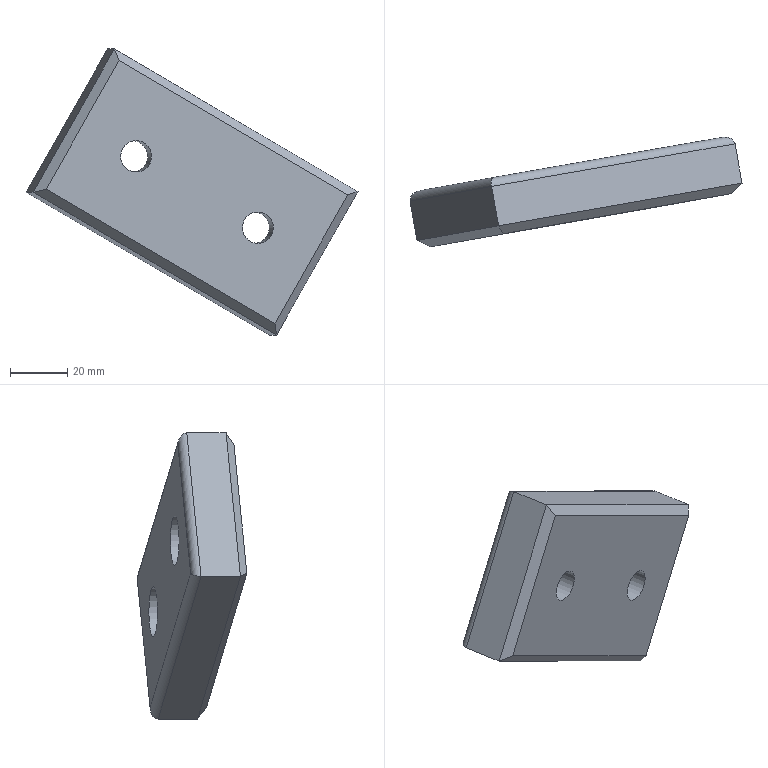Part | NX | features solid 2 | 1 solid | 20 faces | box 116.311 x 38.432 x 100.229 mm | volume 106721 mm3 | plane 12 | cylinder 8 | commonest cylinder face diameters 6 x4 11 x2 17.5 x2
STEP:
#1=CARTESIAN_POINT('',(794.909,638.341,-0.113));
#2=VERTEX_POINT('',#1);
#3=CARTESIAN_POINT('',(792.478,652.128,-0.113));
#4=VERTEX_POINT('',#3);
#5=CARTESIAN_POINT('',(795.43,635.386,-0.113));
#6=DIRECTION('',(-0.1736,0.9848,0.));
#7=VECTOR('',#6,1000.);
#8=LINE('',#5,#7);
#9=EDGE_CURVE('',#2,#4,#8,.T.);
#10=ORIENTED_EDGE('',*,*,#9,.F.);
#11=CARTESIAN_POINT('',(823.469,643.376,50.117));
#12=VERTEX_POINT('',#11);
#13=CARTESIAN_POINT('',(823.469,643.376,50.117));
#14=DIRECTION('',(0.4924,0.08682,0.866));
#15=VECTOR('',#14,1000.);
#16=LINE('',#13,#15);
#17=EDGE_CURVE('',#2,#12,#16,.T.);
#18=ORIENTED_EDGE('',*,*,#17,.T.);
#19=CARTESIAN_POINT('',(821.038,657.164,50.117));
#20=VERTEX_POINT('',#19);
#21=CARTESIAN_POINT('',(823.99,640.422,50.117));
#22=DIRECTION('',(-0.1736,0.9848,0.));
#23=VECTOR('',#22,1000.);
#24=LINE('',#21,#23);
#25=EDGE_CURVE('',#12,#20,#24,.T.);
#26=ORIENTED_EDGE('',*,*,#25,.T.);
#27=CARTESIAN_POINT('',(821.038,657.164,50.117));
#28=DIRECTION('',(-0.4924,-0.08682,-0.866));
#29=VECTOR('',#28,1000.);
#30=LINE('',#27,#29);
#31=EDGE_CURVE('',#20,#4,#30,.T.);
#32=ORIENTED_EDGE('',*,*,#31,.T.);
#33=EDGE_LOOP('',(#10,#18,#26,#32));
#34=FACE_BOUND('',#33,.T.);
#35=CARTESIAN_POINT('',(823.99,640.422,50.117));
#36=DIRECTION('',(0.8529,0.1504,-0.5));
#37=DIRECTION('',(-0.1736,0.9848,0.));
#38=AXIS2_PLACEMENT_3D('',#35,#36,#37);
#39=PLANE('',#38);
#40=ADVANCED_FACE('',(#34),#39,.F.);
#41=CARTESIAN_POINT('',(880.196,653.379,-50.113));
#42=VERTEX_POINT('',#41);
#43=CARTESIAN_POINT('',(877.765,667.166,-50.113));
#44=VERTEX_POINT('',#43);
#45=CARTESIAN_POINT('',(880.717,650.425,-50.113));
#46=DIRECTION('',(-0.1736,0.9848,0.));
#47=VECTOR('',#46,1000.);
#48=LINE('',#45,#47);
#49=EDGE_CURVE('',#42,#44,#48,.T.);
#50=ORIENTED_EDGE('',*,*,#49,.F.);
#51=CARTESIAN_POINT('',(794.909,638.341,-0.113));
#52=DIRECTION('',(-0.8529,-0.1504,0.5));
#53=VECTOR('',#52,1000.);
#54=LINE('',#51,#53);
#55=EDGE_CURVE('',#42,#2,#54,.T.);
#56=ORIENTED_EDGE('',*,*,#55,.T.);
#57=ORIENTED_EDGE('',*,*,#9,.T.);
#58=CARTESIAN_POINT('',(792.478,652.128,-0.113));
#59=DIRECTION('',(0.8529,0.1504,-0.5));
#60=VECTOR('',#59,1000.);
#61=LINE('',#58,#60);
#62=EDGE_CURVE('',#4,#44,#61,.T.);
#63=ORIENTED_EDGE('',*,*,#62,.T.);
#64=EDGE_LOOP('',(#50,#56,#57,#63));
#65=FACE_BOUND('',#64,.T.);
#66=CARTESIAN_POINT('',(795.43,635.386,-0.113));
#67=DIRECTION('',(0.4924,0.08682,0.866));
#68=DIRECTION('',(0.8529,0.1504,-0.5));
#69=AXIS2_PLACEMENT_3D('',#66,#67,#68);
#70=PLANE('',#69);
#71=ADVANCED_FACE('',(#65),#70,.F.);
#72=CARTESIAN_POINT('',(908.756,658.415,0.1165));
#73=VERTEX_POINT('',#72);
#74=CARTESIAN_POINT('',(906.325,672.202,0.1165));
#75=VERTEX_POINT('',#74);
#76=CARTESIAN_POINT('',(909.277,655.46,0.1165));
#77=DIRECTION('',(-0.1736,0.9848,0.));
#78=VECTOR('',#77,1000.);
#79=LINE('',#76,#78);
#80=EDGE_CURVE('',#73,#75,#79,.T.);
#81=ORIENTED_EDGE('',*,*,#80,.F.);
#82=CARTESIAN_POINT('',(880.196,653.379,-50.113));
#83=DIRECTION('',(-0.4924,-0.08682,-0.866));
#84=VECTOR('',#83,1000.);
#85=LINE('',#82,#84);
#86=EDGE_CURVE('',#73,#42,#85,.T.);
#87=ORIENTED_EDGE('',*,*,#86,.T.);
#88=ORIENTED_EDGE('',*,*,#49,.T.);
#89=CARTESIAN_POINT('',(877.765,667.166,-50.113));
#90=DIRECTION('',(0.4924,0.08682,0.866));
#91=VECTOR('',#90,1000.);
#92=LINE('',#89,#91);
#93=EDGE_CURVE('',#44,#75,#92,.T.);
#94=ORIENTED_EDGE('',*,*,#93,.T.);
#95=EDGE_LOOP('',(#81,#87,#88,#94));
#96=FACE_BOUND('',#95,.T.);
#97=CARTESIAN_POINT('',(880.717,650.425,-50.113));
#98=DIRECTION('',(-0.8529,-0.1504,0.5));
#99=DIRECTION('',(0.1736,-0.9848,0.));
#100=AXIS2_PLACEMENT_3D('',#97,#98,#99);
#101=PLANE('',#100);
#102=ADVANCED_FACE('',(#96),#101,.F.);
#103=ORIENTED_EDGE('',*,*,#25,.F.);
#104=CARTESIAN_POINT('',(930.077,662.174,-12.383));
#105=DIRECTION('',(0.8529,0.1504,-0.5));
#106=VECTOR('',#105,1000.);
#107=LINE('',#104,#106);
#108=EDGE_CURVE('',#12,#73,#107,.T.);
#109=ORIENTED_EDGE('',*,*,#108,.T.);
#110=ORIENTED_EDGE('',*,*,#80,.T.);
#111=CARTESIAN_POINT('',(927.646,675.962,-12.383));
#112=DIRECTION('',(-0.8529,-0.1504,0.5));
#113=VECTOR('',#112,1000.);
#114=LINE('',#111,#113);
#115=EDGE_CURVE('',#75,#20,#114,.T.);
#116=ORIENTED_EDGE('',*,*,#115,.T.);
#117=EDGE_LOOP('',(#103,#109,#110,#116));
#118=FACE_BOUND('',#117,.T.);
#119=CARTESIAN_POINT('',(930.598,659.22,-12.383));
#120=DIRECTION('',(-0.4924,-0.08682,-0.866));
#121=DIRECTION('',(-0.8529,-0.1504,0.5));
#122=AXIS2_PLACEMENT_3D('',#119,#120,#121);
#123=PLANE('',#122);
#124=ADVANCED_FACE('',(#118),#123,.F.);
#125=CARTESIAN_POINT('',(799.466,636.098,0.9851));
#126=VERTEX_POINT('',#125);
#127=CARTESIAN_POINT('',(879.636,650.234,-46.015));
#128=VERTEX_POINT('',#127);
#129=CARTESIAN_POINT('',(903.516,654.445,-60.015));
#130=DIRECTION('',(0.8529,0.1504,-0.5));
#131=VECTOR('',#130,1000.);
#132=LINE('',#129,#131);
#133=EDGE_CURVE('',#126,#128,#132,.T.);
#134=ORIENTED_EDGE('',*,*,#133,.T.);
#135=CARTESIAN_POINT('',(905.241,654.749,-0.9816));
#136=VERTEX_POINT('',#135);
#137=CARTESIAN_POINT('',(906.718,655.009,1.617));
#138=DIRECTION('',(0.4924,0.08682,0.866));
#139=VECTOR('',#138,1000.);
#140=LINE('',#137,#139);
#141=EDGE_CURVE('',#128,#136,#140,.T.);
#142=ORIENTED_EDGE('',*,*,#141,.T.);
#143=CARTESIAN_POINT('',(825.071,640.613,46.018));
#144=VERTEX_POINT('',#143);
#145=CARTESIAN_POINT('',(822.513,640.162,47.518));
#146=DIRECTION('',(-0.8529,-0.1504,0.5));
#147=VECTOR('',#146,1000.);
#148=LINE('',#145,#147);
#149=EDGE_CURVE('',#136,#144,#148,.T.);
#150=ORIENTED_EDGE('',*,*,#149,.T.);
#151=CARTESIAN_POINT('',(797.989,635.837,-1.613));
#152=DIRECTION('',(-0.4924,-0.08682,-0.866));
#153=VECTOR('',#152,1000.);
#154=LINE('',#151,#153);
#155=EDGE_CURVE('',#144,#126,#154,.T.);
#156=ORIENTED_EDGE('',*,*,#155,.T.);
#157=EDGE_LOOP('',(#134,#142,#150,#156));
#158=FACE_BOUND('',#157,.T.);
#159=CARTESIAN_POINT('',(878.366,650.01,-15.248));
#160=VERTEX_POINT('',#159);
#161=CARTESIAN_POINT('',(873.675,649.183,-12.498));
#162=DIRECTION('',(0.1736,-0.9848,0.));
#163=DIRECTION('',(0.8529,0.1504,-0.5));
#164=AXIS2_PLACEMENT_3D('',#161,#162,#163);
#165=CIRCLE('',#164,5.5);
#166=EDGE_CURVE('',#160,#160,#165,.T.);
#167=ORIENTED_EDGE('',*,*,#166,.F.);
#168=EDGE_LOOP('',(#167));
#169=FACE_BOUND('',#168,.T.);
#170=CARTESIAN_POINT('',(835.722,642.491,9.752));
#171=VERTEX_POINT('',#170);
#172=CARTESIAN_POINT('',(831.032,641.664,12.502));
#173=DIRECTION('',(0.1736,-0.9848,0.));
#174=DIRECTION('',(0.8529,0.1504,-0.5));
#175=AXIS2_PLACEMENT_3D('',#172,#173,#174);
#176=CIRCLE('',#175,5.5);
#177=EDGE_CURVE('',#171,#171,#176,.T.);
#178=ORIENTED_EDGE('',*,*,#177,.F.);
#179=EDGE_LOOP('',(#178));
#180=FACE_BOUND('',#179,.T.);
#181=CARTESIAN_POINT('',(795.43,635.386,-0.113));
#182=DIRECTION('',(0.1736,-0.9848,0.));
#183=DIRECTION('',(0.8529,0.1504,-0.5));
#184=AXIS2_PLACEMENT_3D('',#181,#182,#183);
#185=PLANE('',#184);
#186=ADVANCED_FACE('',(#158,#169,#180),#185,.T.);
#187=CARTESIAN_POINT('',(795.993,655.794,0.9851));
#188=VERTEX_POINT('',#187);
#189=CARTESIAN_POINT('',(821.598,660.309,46.018));
#190=VERTEX_POINT('',#189);
#191=CARTESIAN_POINT('',(794.516,655.534,-1.613));
#192=DIRECTION('',(-0.4924,-0.08682,-0.866));
#193=VECTOR('',#192,1000.);
#194=LINE('',#191,#193);
#195=EDGE_CURVE('',#188,#190,#194,.F.);
#196=ORIENTED_EDGE('',*,*,#195,.T.);
#197=CARTESIAN_POINT('',(901.768,674.445,-0.9816));
#198=VERTEX_POINT('',#197);
#199=CARTESIAN_POINT('',(819.04,659.858,47.518));
#200=DIRECTION('',(-0.8529,-0.1504,0.5));
#201=VECTOR('',#200,1000.);
#202=LINE('',#199,#201);
#203=EDGE_CURVE('',#190,#198,#202,.F.);
#204=ORIENTED_EDGE('',*,*,#203,.T.);
#205=CARTESIAN_POINT('',(876.163,669.93,-46.015));
#206=VERTEX_POINT('',#205);
#207=CARTESIAN_POINT('',(874.686,669.67,-48.613));
#208=DIRECTION('',(0.4924,0.08682,0.866));
#209=VECTOR('',#208,1000.);
#210=LINE('',#207,#209);
#211=EDGE_CURVE('',#198,#206,#210,.F.);
#212=ORIENTED_EDGE('',*,*,#211,.T.);
#213=CARTESIAN_POINT('',(793.435,655.343,2.485));
#214=DIRECTION('',(0.8529,0.1504,-0.5));
#215=VECTOR('',#214,1000.);
#216=LINE('',#213,#215);
#217=EDGE_CURVE('',#206,#188,#216,.F.);
#218=ORIENTED_EDGE('',*,*,#217,.T.);
#219=EDGE_LOOP('',(#196,#204,#212,#218));
#220=FACE_BOUND('',#219,.T.);
#221=CARTESIAN_POINT('',(877.665,670.195,-16.873));
#222=VERTEX_POINT('',#221);
#223=CARTESIAN_POINT('',(870.202,668.879,-12.498));
#224=DIRECTION('',(0.1736,-0.9848,0.));
#225=DIRECTION('',(0.8529,0.1504,-0.5));
#226=AXIS2_PLACEMENT_3D('',#223,#224,#225);
#227=CIRCLE('',#226,8.75);
#228=EDGE_CURVE('',#222,#222,#227,.T.);
#229=ORIENTED_EDGE('',*,*,#228,.T.);
#230=EDGE_LOOP('',(#229));
#231=FACE_BOUND('',#230,.T.);
#232=CARTESIAN_POINT('',(835.021,662.676,8.127));
#233=VERTEX_POINT('',#232);
#234=CARTESIAN_POINT('',(827.559,661.36,12.502));
#235=DIRECTION('',(0.1736,-0.9848,0.));
#236=DIRECTION('',(0.8529,0.1504,-0.5));
#237=AXIS2_PLACEMENT_3D('',#234,#235,#236);
#238=CIRCLE('',#237,8.75);
#239=EDGE_CURVE('',#233,#233,#238,.T.);
#240=ORIENTED_EDGE('',*,*,#239,.T.);
#241=EDGE_LOOP('',(#240));
#242=FACE_BOUND('',#241,.T.);
#243=CARTESIAN_POINT('',(791.957,655.082,-0.113));
#244=DIRECTION('',(0.1736,-0.9848,0.));
#245=DIRECTION('',(0.8529,0.1504,-0.5));
#246=AXIS2_PLACEMENT_3D('',#243,#244,#245);
#247=PLANE('',#246);
#248=ADVANCED_FACE('',(#220,#231,#242),#247,.F.);
#249=ORIENTED_EDGE('',*,*,#177,.T.);
#250=EDGE_LOOP('',(#249));
#251=FACE_BOUND('',#250,.T.);
#252=CARTESIAN_POINT('',(834.333,650.369,9.752));
#253=VERTEX_POINT('',#252);
#254=CARTESIAN_POINT('',(829.643,649.542,12.502));
#255=DIRECTION('',(0.1736,-0.9848,0.));
#256=DIRECTION('',(0.8529,0.1504,-0.5));
#257=AXIS2_PLACEMENT_3D('',#254,#255,#256);
#258=CIRCLE('',#257,5.5);
#259=EDGE_CURVE('',#253,#253,#258,.T.);
#260=ORIENTED_EDGE('',*,*,#259,.F.);
#261=EDGE_LOOP('',(#260));
#262=FACE_BOUND('',#261,.T.);
#263=CARTESIAN_POINT('',(836.241,612.119,12.502));
#264=DIRECTION('',(0.1736,-0.9848,0.));
#265=DIRECTION('',(0.8529,0.1504,-0.5));
#266=AXIS2_PLACEMENT_3D('',#263,#264,#265);
#267=CYLINDRICAL_SURFACE('',#266,5.5);
#268=ADVANCED_FACE('',(#251,#262),#267,.F.);
#269=ORIENTED_EDGE('',*,*,#259,.T.);
#270=EDGE_LOOP('',(#269));
#271=FACE_BOUND('',#270,.T.);
#272=CARTESIAN_POINT('',(837.105,650.858,8.127));
#273=VERTEX_POINT('',#272);
#274=CARTESIAN_POINT('',(829.643,649.542,12.502));
#275=DIRECTION('',(0.1736,-0.9848,0.));
#276=DIRECTION('',(0.8529,0.1504,-0.5));
#277=AXIS2_PLACEMENT_3D('',#274,#275,#276);
#278=CIRCLE('',#277,8.75);
#279=EDGE_CURVE('',#273,#273,#278,.T.);
#280=ORIENTED_EDGE('',*,*,#279,.F.);
#281=EDGE_LOOP('',(#280));
#282=FACE_BOUND('',#281,.T.);
#283=CARTESIAN_POINT('',(829.643,649.542,12.502));
#284=DIRECTION('',(0.1736,-0.9848,0.));
#285=DIRECTION('',(0.8529,0.1504,-0.5));
#286=AXIS2_PLACEMENT_3D('',#283,#284,#285);
#287=PLANE('',#286);
#288=ADVANCED_FACE('',(#271,#282),#287,.F.);
#289=ORIENTED_EDGE('',*,*,#279,.T.);
#290=EDGE_LOOP('',(#289));
#291=FACE_BOUND('',#290,.T.);
#292=ORIENTED_EDGE('',*,*,#239,.F.);
#293=EDGE_LOOP('',(#292));
#294=FACE_BOUND('',#293,.T.);
#295=CARTESIAN_POINT('',(827.559,661.36,12.502));
#296=DIRECTION('',(0.1736,-0.9848,0.));
#297=DIRECTION('',(0.8529,0.1504,-0.5));
#298=AXIS2_PLACEMENT_3D('',#295,#296,#297);
#299=CYLINDRICAL_SURFACE('',#298,8.75);
#300=ADVANCED_FACE('',(#291,#294),#299,.F.);
#301=ORIENTED_EDGE('',*,*,#166,.T.);
#302=EDGE_LOOP('',(#301));
#303=FACE_BOUND('',#302,.T.);
#304=CARTESIAN_POINT('',(876.977,657.888,-15.248));
#305=VERTEX_POINT('',#304);
#306=CARTESIAN_POINT('',(872.286,657.061,-12.498));
#307=DIRECTION('',(0.1736,-0.9848,0.));
#308=DIRECTION('',(0.8529,0.1504,-0.5));
#309=AXIS2_PLACEMENT_3D('',#306,#307,#308);
#310=CIRCLE('',#309,5.5);
#311=EDGE_CURVE('',#305,#305,#310,.T.);
#312=ORIENTED_EDGE('',*,*,#311,.F.);
#313=EDGE_LOOP('',(#312));
#314=FACE_BOUND('',#313,.T.);
#315=CARTESIAN_POINT('',(878.885,619.639,-12.498));
#316=DIRECTION('',(0.1736,-0.9848,0.));
#317=DIRECTION('',(0.8529,0.1504,-0.5));
#318=AXIS2_PLACEMENT_3D('',#315,#316,#317);
#319=CYLINDRICAL_SURFACE('',#318,5.5);
#320=ADVANCED_FACE('',(#303,#314),#319,.F.);
#321=ORIENTED_EDGE('',*,*,#311,.T.);
#322=EDGE_LOOP('',(#321));
#323=FACE_BOUND('',#322,.T.);
#324=CARTESIAN_POINT('',(879.749,658.377,-16.873));
#325=VERTEX_POINT('',#324);
#326=CARTESIAN_POINT('',(872.286,657.061,-12.498));
#327=DIRECTION('',(0.1736,-0.9848,0.));
#328=DIRECTION('',(0.8529,0.1504,-0.5));
#329=AXIS2_PLACEMENT_3D('',#326,#327,#328);
#330=CIRCLE('',#329,8.75);
#331=EDGE_CURVE('',#325,#325,#330,.T.);
#332=ORIENTED_EDGE('',*,*,#331,.F.);
#333=EDGE_LOOP('',(#332));
#334=FACE_BOUND('',#333,.T.);
#335=CARTESIAN_POINT('',(872.286,657.061,-12.498));
#336=DIRECTION('',(0.1736,-0.9848,0.));
#337=DIRECTION('',(0.8529,0.1504,-0.5));
#338=AXIS2_PLACEMENT_3D('',#335,#336,#337);
#339=PLANE('',#338);
#340=ADVANCED_FACE('',(#323,#334),#339,.F.);
#341=ORIENTED_EDGE('',*,*,#331,.T.);
#342=EDGE_LOOP('',(#341));
#343=FACE_BOUND('',#342,.T.);
#344=ORIENTED_EDGE('',*,*,#228,.F.);
#345=EDGE_LOOP('',(#344));
#346=FACE_BOUND('',#345,.T.);
#347=CARTESIAN_POINT('',(870.202,668.879,-12.498));
#348=DIRECTION('',(0.1736,-0.9848,0.));
#349=DIRECTION('',(0.8529,0.1504,-0.5));
#350=AXIS2_PLACEMENT_3D('',#347,#348,#349);
#351=CYLINDRICAL_SURFACE('',#350,8.75);
#352=ADVANCED_FACE('',(#343,#346),#351,.F.);
#353=CARTESIAN_POINT('',(796.514,652.84,0.9851));
#354=DIRECTION('',(0.2549,0.04494,-0.9659));
#355=DIRECTION('',(-0.9513,-0.1677,-0.2588));
#356=AXIS2_PLACEMENT_3D('',#353,#354,#355);
#357=ELLIPSE('',#356,4.243,3.);
#358=EDGE_CURVE('',#188,#4,#357,.F.);
#359=ORIENTED_EDGE('',*,*,#358,.F.);
#360=ORIENTED_EDGE('',*,*,#217,.F.);
#361=CARTESIAN_POINT('',(876.684,666.976,-46.015));
#362=DIRECTION('',(0.9513,0.1677,0.2588));
#363=DIRECTION('',(0.2549,0.04494,-0.9659));
#364=AXIS2_PLACEMENT_3D('',#361,#362,#363);
#365=ELLIPSE('',#364,4.243,3.);
#366=EDGE_CURVE('',#44,#206,#365,.T.);
#367=ORIENTED_EDGE('',*,*,#366,.F.);
#368=ORIENTED_EDGE('',*,*,#62,.F.);
#369=EDGE_LOOP('',(#359,#360,#367,#368));
#370=FACE_BOUND('',#369,.T.);
#371=CARTESIAN_POINT('',(793.955,652.388,2.485));
#372=DIRECTION('',(0.8529,0.1504,-0.5));
#373=DIRECTION('',(-0.1736,0.9848,0.));
#374=AXIS2_PLACEMENT_3D('',#371,#372,#373);
#375=CYLINDRICAL_SURFACE('',#374,3.);
#376=ADVANCED_FACE('',(#370),#375,.T.);
#377=ORIENTED_EDGE('',*,*,#366,.T.);
#378=ORIENTED_EDGE('',*,*,#211,.F.);
#379=CARTESIAN_POINT('',(902.289,671.491,-0.9816));
#380=DIRECTION('',(-0.2549,-0.04494,0.9659));
#381=DIRECTION('',(0.9513,0.1677,0.2588));
#382=AXIS2_PLACEMENT_3D('',#379,#380,#381);
#383=ELLIPSE('',#382,4.243,3.);
#384=EDGE_CURVE('',#75,#198,#383,.T.);
#385=ORIENTED_EDGE('',*,*,#384,.F.);
#386=ORIENTED_EDGE('',*,*,#93,.F.);
#387=EDGE_LOOP('',(#377,#378,#385,#386));
#388=FACE_BOUND('',#387,.T.);
#389=CARTESIAN_POINT('',(875.207,666.715,-48.613));
#390=DIRECTION('',(0.4924,0.08682,0.866));
#391=DIRECTION('',(0.8529,0.1504,-0.5));
#392=AXIS2_PLACEMENT_3D('',#389,#390,#391);
#393=CYLINDRICAL_SURFACE('',#392,3.);
#394=ADVANCED_FACE('',(#388),#393,.T.);
#395=ORIENTED_EDGE('',*,*,#358,.T.);
#396=ORIENTED_EDGE('',*,*,#31,.F.);
#397=CARTESIAN_POINT('',(822.119,657.354,46.018));
#398=DIRECTION('',(-0.9513,-0.1677,-0.2588));
#399=DIRECTION('',(0.2549,0.04494,-0.9659));
#400=AXIS2_PLACEMENT_3D('',#397,#398,#399);
#401=ELLIPSE('',#400,4.243,3.);
#402=EDGE_CURVE('',#190,#20,#401,.F.);
#403=ORIENTED_EDGE('',*,*,#402,.F.);
#404=ORIENTED_EDGE('',*,*,#195,.F.);
#405=EDGE_LOOP('',(#395,#396,#403,#404));
#406=FACE_BOUND('',#405,.T.);
#407=CARTESIAN_POINT('',(823.596,657.615,48.617));
#408=DIRECTION('',(-0.4924,-0.08682,-0.866));
#409=DIRECTION('',(-0.8529,-0.1504,0.5));
#410=AXIS2_PLACEMENT_3D('',#407,#408,#409);
#411=CYLINDRICAL_SURFACE('',#410,3.);
#412=ADVANCED_FACE('',(#406),#411,.T.);
#413=ORIENTED_EDGE('',*,*,#384,.T.);
#414=ORIENTED_EDGE('',*,*,#203,.F.);
#415=ORIENTED_EDGE('',*,*,#402,.T.);
#416=ORIENTED_EDGE('',*,*,#115,.F.);
#417=EDGE_LOOP('',(#413,#414,#415,#416));
#418=FACE_BOUND('',#417,.T.);
#419=CARTESIAN_POINT('',(926.169,675.701,-14.982));
#420=DIRECTION('',(-0.8529,-0.1504,0.5));
#421=DIRECTION('',(0.4924,0.08682,0.866));
#422=AXIS2_PLACEMENT_3D('',#419,#420,#421);
#423=CYLINDRICAL_SURFACE('',#422,3.);
#424=ADVANCED_FACE('',(#418),#423,.T.);
#425=CARTESIAN_POINT('',(824.537,641.534,47.384));
#426=DIRECTION('',(0.3084,-0.5319,-0.7887));
#427=VECTOR('',#426,1000.);
#428=LINE('',#425,#427);
#429=EDGE_CURVE('',#12,#144,#428,.T.);
#430=ORIENTED_EDGE('',*,*,#429,.F.);
#431=ORIENTED_EDGE('',*,*,#17,.F.);
#432=CARTESIAN_POINT('',(797.947,636.845,0.6191));
#433=DIRECTION('',(0.8769,-0.4316,0.2113));
#434=VECTOR('',#433,1000.);
#435=LINE('',#432,#434);
#436=EDGE_CURVE('',#126,#2,#435,.F.);
#437=ORIENTED_EDGE('',*,*,#436,.F.);
#438=ORIENTED_EDGE('',*,*,#155,.F.);
#439=EDGE_LOOP('',(#430,#431,#437,#438));
#440=FACE_BOUND('',#439,.T.);
#441=CARTESIAN_POINT('',(797.989,635.837,-1.613));
#442=DIRECTION('',(-0.4803,-0.8027,0.3536));
#443=DIRECTION('',(0.7259,-0.59,-0.3536));
#444=AXIS2_PLACEMENT_3D('',#441,#442,#443);
#445=PLANE('',#444);
#446=ADVANCED_FACE('',(#440),#445,.T.);
#447=ORIENTED_EDGE('',*,*,#436,.T.);
#448=ORIENTED_EDGE('',*,*,#55,.F.);
#449=CARTESIAN_POINT('',(872.039,607.6,9.537));
#450=DIRECTION('',(-0.1079,-0.6053,0.7887));
#451=VECTOR('',#450,1000.);
#452=LINE('',#449,#451);
#453=EDGE_CURVE('',#128,#42,#452,.F.);
#454=ORIENTED_EDGE('',*,*,#453,.F.);
#455=ORIENTED_EDGE('',*,*,#133,.F.);
#456=EDGE_LOOP('',(#447,#448,#454,#455));
#457=FACE_BOUND('',#456,.T.);
#458=CARTESIAN_POINT('',(796.908,635.647,2.485));
#459=DIRECTION('',(-0.2254,-0.7578,-0.6124));
#460=DIRECTION('',(-0.471,0.635,-0.6124));
#461=AXIS2_PLACEMENT_3D('',#458,#459,#460);
#462=PLANE('',#461);
#463=ADVANCED_FACE('',(#457),#462,.T.);
#464=ORIENTED_EDGE('',*,*,#429,.T.);
#465=ORIENTED_EDGE('',*,*,#149,.F.);
#466=CARTESIAN_POINT('',(857.595,605.053,-15.867));
#467=DIRECTION('',(0.6764,0.7055,0.2113));
#468=VECTOR('',#467,1000.);
#469=LINE('',#466,#468);
#470=EDGE_CURVE('',#73,#136,#469,.F.);
#471=ORIENTED_EDGE('',*,*,#470,.F.);
#472=ORIENTED_EDGE('',*,*,#108,.F.);
#473=EDGE_LOOP('',(#464,#465,#471,#472));
#474=FACE_BOUND('',#473,.T.);
#475=CARTESIAN_POINT('',(822.513,640.162,47.518));
#476=DIRECTION('',(0.471,-0.635,0.6124));
#477=DIRECTION('',(-0.2254,-0.7578,-0.6124));
#478=AXIS2_PLACEMENT_3D('',#475,#476,#477);
#479=PLANE('',#478);
#480=ADVANCED_FACE('',(#474),#479,.T.);
#481=ORIENTED_EDGE('',*,*,#453,.T.);
#482=ORIENTED_EDGE('',*,*,#86,.F.);
#483=ORIENTED_EDGE('',*,*,#470,.T.);
#484=ORIENTED_EDGE('',*,*,#141,.F.);
#485=EDGE_LOOP('',(#481,#482,#483,#484));
#486=FACE_BOUND('',#485,.T.);
#487=CARTESIAN_POINT('',(878.159,649.973,-48.613));
#488=DIRECTION('',(0.7259,-0.59,-0.3536));
#489=DIRECTION('',(0.4803,0.8027,-0.3536));
#490=AXIS2_PLACEMENT_3D('',#487,#488,#489);
#491=PLANE('',#490);
#492=ADVANCED_FACE('',(#486),#491,.T.);
#493=CLOSED_SHELL('',(#40,#71,#102,#124,#186,#248,#268,#288,#300,#320,#340,#352,#376,#394,#412,#424,#446,#463,#480,#492));
#494=MANIFOLD_SOLID_BREP('',#493);
#495=(LENGTH_UNIT()NAMED_UNIT(*)SI_UNIT(.MILLI.,.METRE.));
#496=UNCERTAINTY_MEASURE_WITH_UNIT(LENGTH_MEASURE(0.00001),#495,'','');
#497=(NAMED_UNIT(*)PLANE_ANGLE_UNIT()SI_UNIT($,.RADIAN.));
#498=(NAMED_UNIT(*)SI_UNIT($,.STERADIAN.)SOLID_ANGLE_UNIT());
#499=(GEOMETRIC_REPRESENTATION_CONTEXT(3)GLOBAL_UNCERTAINTY_ASSIGNED_CONTEXT((#496))GLOBAL_UNIT_ASSIGNED_CONTEXT((#495,#497,#498))REPRESENTATION_CONTEXT('',''));
#500=ADVANCED_BREP_SHAPE_REPRESENTATION('',(#494),#499);